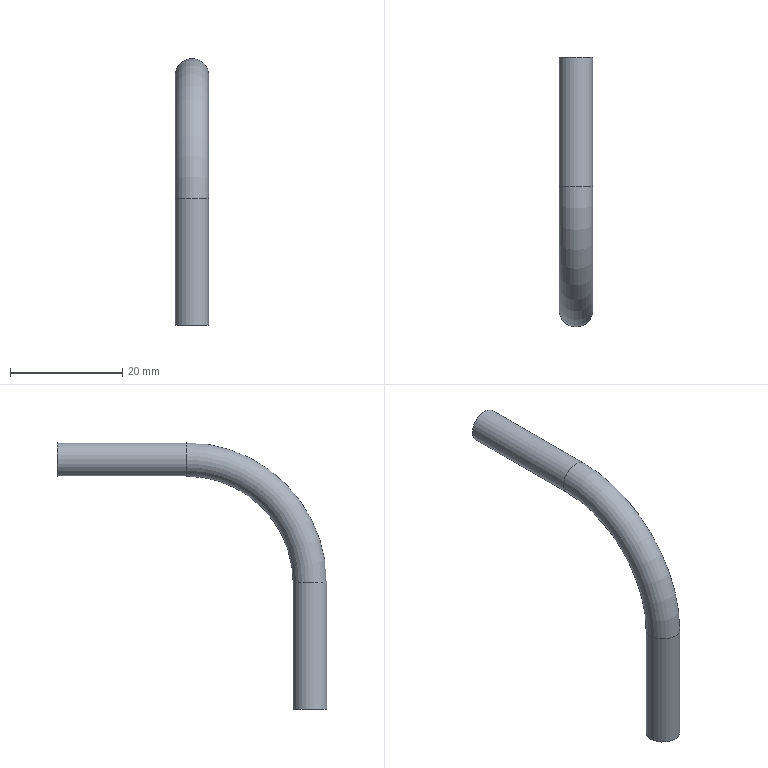Part | STEP file | 1-51.3 | 1 solid | 8 faces | box 6 x 48 x 47.5 mm | volume 691.647 mm3 | cylinder 4 | torus 2 | plane 2 | commonest cylinder face diameters 5 x2 6 x2
STEP:
#1=CARTESIAN_POINT('',(0.,0.,0.));
#2=DIRECTION('',(0.,0.,1.));
#3=DIRECTION('',(1.,0.,0.));
#4=AXIS2_PLACEMENT_3D('',#1,#2,#3);
#5=CARTESIAN_POINT('',(3.,0.,0.));
#6=VERTEX_POINT('',#5);
#7=CARTESIAN_POINT('',(0.,0.,0.));
#8=DIRECTION('',(0.,0.,-1.));
#9=DIRECTION('',(1.,0.,0.));
#10=AXIS2_PLACEMENT_3D('',#7,#8,#9);
#11=CIRCLE('',#10,3.);
#12=CARTESIAN_POINT('',(0.,0.,0.));
#13=DIRECTION('',(0.,0.,1.));
#14=DIRECTION('',(1.,0.,0.));
#15=AXIS2_PLACEMENT_3D('',#12,#13,#14);
#16=CYLINDRICAL_SURFACE('',#15,3.);
#17=CARTESIAN_POINT('',(6.283,0.));
#18=DIRECTION('',(-1.,0.));
#19=VECTOR('',#18,1.);
#20=LINE('',#17,#19);
#21=(GEOMETRIC_REPRESENTATION_CONTEXT(2)PARAMETRIC_REPRESENTATION_CONTEXT()REPRESENTATION_CONTEXT('',''));
#22=DEFINITIONAL_REPRESENTATION('',(#20),#21);
#23=PCURVE('',#16,#22);
#24=CARTESIAN_POINT('',(0.,0.,0.));
#25=DIRECTION('',(0.,0.,-1.));
#26=DIRECTION('',(1.,0.,0.));
#27=AXIS2_PLACEMENT_3D('',#24,#25,#26);
#28=PLANE('',#27);
#29=CARTESIAN_POINT('',(0.,0.));
#30=DIRECTION('',(1.,0.));
#31=AXIS2_PLACEMENT_2D('',#29,#30);
#32=CIRCLE('',#31,3.);
#33=(GEOMETRIC_REPRESENTATION_CONTEXT(2)PARAMETRIC_REPRESENTATION_CONTEXT()REPRESENTATION_CONTEXT('',''));
#34=DEFINITIONAL_REPRESENTATION('',(#32),#33);
#35=PCURVE('',#28,#34);
#36=SURFACE_CURVE('',#11,(#23,#35),.PCURVE_S1.);
#37=EDGE_CURVE('',#6,#6,#36,.T.);
#38=ORIENTED_EDGE('',*,*,#37,.F.);
#39=CARTESIAN_POINT('',(3.,0.,22.5));
#40=VERTEX_POINT('',#39);
#41=CARTESIAN_POINT('',(3.,0.,0.));
#42=DIRECTION('',(0.,0.,1.));
#43=VECTOR('',#42,1.);
#44=LINE('',#41,#43);
#45=CARTESIAN_POINT('',(6.283,0.));
#46=DIRECTION('',(0.,1.));
#47=VECTOR('',#46,1.);
#48=LINE('',#45,#47);
#49=(GEOMETRIC_REPRESENTATION_CONTEXT(2)PARAMETRIC_REPRESENTATION_CONTEXT()REPRESENTATION_CONTEXT('',''));
#50=DEFINITIONAL_REPRESENTATION('',(#48),#49);
#51=PCURVE('',#16,#50);
#52=CARTESIAN_POINT('',(0.,0.));
#53=DIRECTION('',(0.,1.));
#54=VECTOR('',#53,1.);
#55=LINE('',#52,#54);
#56=(GEOMETRIC_REPRESENTATION_CONTEXT(2)PARAMETRIC_REPRESENTATION_CONTEXT()REPRESENTATION_CONTEXT('',''));
#57=DEFINITIONAL_REPRESENTATION('',(#55),#56);
#58=PCURVE('',#16,#57);
#59=SEAM_CURVE('',#44,(#51,#58),.PCURVE_S1.);
#60=EDGE_CURVE('',#6,#40,#59,.T.);
#61=ORIENTED_EDGE('',*,*,#60,.T.);
#62=CARTESIAN_POINT('',(-3.,0.,22.5));
#63=VERTEX_POINT('',#62);
#64=CARTESIAN_POINT('',(0.,0.,22.5));
#65=DIRECTION('',(0.,0.,1.));
#66=DIRECTION('',(-1.,0.,0.));
#67=AXIS2_PLACEMENT_3D('',#64,#65,#66);
#68=CIRCLE('',#67,3.);
#69=CARTESIAN_POINT('',(3.142,22.5));
#70=DIRECTION('',(1.,0.));
#71=VECTOR('',#70,1.);
#72=LINE('',#69,#71);
#73=(GEOMETRIC_REPRESENTATION_CONTEXT(2)PARAMETRIC_REPRESENTATION_CONTEXT()REPRESENTATION_CONTEXT('',''));
#74=DEFINITIONAL_REPRESENTATION('',(#72),#73);
#75=PCURVE('',#16,#74);
#76=CARTESIAN_POINT('',(0.,22.,22.5));
#77=DIRECTION('',(1.,0.,0.));
#78=DIRECTION('',(0.,-1.,0.));
#79=AXIS2_PLACEMENT_3D('',#76,#77,#78);
#80=TOROIDAL_SURFACE('',#79,22.,3.);
#81=CARTESIAN_POINT('',(6.283,-1.571));
#82=DIRECTION('',(0.,1.));
#83=VECTOR('',#82,1.);
#84=LINE('',#81,#83);
#85=(GEOMETRIC_REPRESENTATION_CONTEXT(2)PARAMETRIC_REPRESENTATION_CONTEXT()REPRESENTATION_CONTEXT('',''));
#86=DEFINITIONAL_REPRESENTATION('',(#84),#85);
#87=PCURVE('',#80,#86);
#88=SURFACE_CURVE('',#68,(#75,#87),.PCURVE_S1.);
#89=EDGE_CURVE('',#63,#40,#88,.T.);
#90=ORIENTED_EDGE('',*,*,#89,.F.);
#91=CARTESIAN_POINT('',(0.,0.,22.5));
#92=DIRECTION('',(0.,0.,1.));
#93=DIRECTION('',(1.,0.,0.));
#94=AXIS2_PLACEMENT_3D('',#91,#92,#93);
#95=CIRCLE('',#94,3.);
#96=CARTESIAN_POINT('',(0.,22.5));
#97=DIRECTION('',(1.,0.));
#98=VECTOR('',#97,1.);
#99=LINE('',#96,#98);
#100=(GEOMETRIC_REPRESENTATION_CONTEXT(2)PARAMETRIC_REPRESENTATION_CONTEXT()REPRESENTATION_CONTEXT('',''));
#101=DEFINITIONAL_REPRESENTATION('',(#99),#100);
#102=PCURVE('',#16,#101);
#103=CARTESIAN_POINT('',(6.283,1.571));
#104=DIRECTION('',(0.,1.));
#105=VECTOR('',#104,1.);
#106=LINE('',#103,#105);
#107=(GEOMETRIC_REPRESENTATION_CONTEXT(2)PARAMETRIC_REPRESENTATION_CONTEXT()REPRESENTATION_CONTEXT('',''));
#108=DEFINITIONAL_REPRESENTATION('',(#106),#107);
#109=PCURVE('',#80,#108);
#110=SURFACE_CURVE('',#95,(#102,#109),.PCURVE_S1.);
#111=EDGE_CURVE('',#40,#63,#110,.T.);
#112=ORIENTED_EDGE('',*,*,#111,.F.);
#113=ORIENTED_EDGE('',*,*,#60,.F.);
#114=EDGE_LOOP('',(#38,#61,#90,#112,#113));
#115=FACE_BOUND('',#114,.T.);
#116=ADVANCED_FACE('',(#115),#16,.T.);
#117=ORIENTED_EDGE('',*,*,#89,.T.);
#118=ORIENTED_EDGE('',*,*,#111,.T.);
#119=CARTESIAN_POINT('',(-3.,22.,44.5));
#120=VERTEX_POINT('',#119);
#121=CARTESIAN_POINT('',(-3.,22.,22.5));
#122=DIRECTION('',(-1.,0.,0.));
#123=DIRECTION('',(0.,-1.,0.));
#124=AXIS2_PLACEMENT_3D('',#121,#122,#123);
#125=CIRCLE('',#124,22.);
#126=CARTESIAN_POINT('',(6.283,4.712));
#127=DIRECTION('',(-1.,0.));
#128=VECTOR('',#127,1.);
#129=LINE('',#126,#128);
#130=(GEOMETRIC_REPRESENTATION_CONTEXT(2)PARAMETRIC_REPRESENTATION_CONTEXT()REPRESENTATION_CONTEXT('',''));
#131=DEFINITIONAL_REPRESENTATION('',(#129),#130);
#132=PCURVE('',#80,#131);
#133=CARTESIAN_POINT('',(6.283,-1.571));
#134=DIRECTION('',(-1.,0.));
#135=VECTOR('',#134,1.);
#136=LINE('',#133,#135);
#137=(GEOMETRIC_REPRESENTATION_CONTEXT(2)PARAMETRIC_REPRESENTATION_CONTEXT()REPRESENTATION_CONTEXT('',''));
#138=DEFINITIONAL_REPRESENTATION('',(#136),#137);
#139=PCURVE('',#80,#138);
#140=SEAM_CURVE('',#125,(#132,#139),.PCURVE_S1.);
#141=EDGE_CURVE('',#63,#120,#140,.T.);
#142=ORIENTED_EDGE('',*,*,#141,.T.);
#143=CARTESIAN_POINT('',(3.,22.,44.5));
#144=VERTEX_POINT('',#143);
#145=CARTESIAN_POINT('',(0.,22.,44.5));
#146=DIRECTION('',(0.,-1.,0.));
#147=DIRECTION('',(-1.,0.,0.));
#148=AXIS2_PLACEMENT_3D('',#145,#146,#147);
#149=CIRCLE('',#148,3.);
#150=CARTESIAN_POINT('',(4.712,4.712));
#151=DIRECTION('',(0.,-1.));
#152=VECTOR('',#151,1.);
#153=LINE('',#150,#152);
#154=(GEOMETRIC_REPRESENTATION_CONTEXT(2)PARAMETRIC_REPRESENTATION_CONTEXT()REPRESENTATION_CONTEXT('',''));
#155=DEFINITIONAL_REPRESENTATION('',(#153),#154);
#156=PCURVE('',#80,#155);
#157=CARTESIAN_POINT('',(0.,22.,44.5));
#158=DIRECTION('',(0.,1.,0.));
#159=DIRECTION('',(1.,0.,0.));
#160=AXIS2_PLACEMENT_3D('',#157,#158,#159);
#161=CYLINDRICAL_SURFACE('',#160,3.);
#162=CARTESIAN_POINT('',(3.142,0.));
#163=DIRECTION('',(-1.,0.));
#164=VECTOR('',#163,1.);
#165=LINE('',#162,#164);
#166=(GEOMETRIC_REPRESENTATION_CONTEXT(2)PARAMETRIC_REPRESENTATION_CONTEXT()REPRESENTATION_CONTEXT('',''));
#167=DEFINITIONAL_REPRESENTATION('',(#165),#166);
#168=PCURVE('',#161,#167);
#169=SURFACE_CURVE('',#149,(#156,#168),.PCURVE_S1.);
#170=EDGE_CURVE('',#120,#144,#169,.T.);
#171=ORIENTED_EDGE('',*,*,#170,.T.);
#172=CARTESIAN_POINT('',(0.,22.,44.5));
#173=DIRECTION('',(0.,-1.,0.));
#174=DIRECTION('',(1.,0.,0.));
#175=AXIS2_PLACEMENT_3D('',#172,#173,#174);
#176=CIRCLE('',#175,3.);
#177=CARTESIAN_POINT('',(4.712,1.571));
#178=DIRECTION('',(0.,-1.));
#179=VECTOR('',#178,1.);
#180=LINE('',#177,#179);
#181=(GEOMETRIC_REPRESENTATION_CONTEXT(2)PARAMETRIC_REPRESENTATION_CONTEXT()REPRESENTATION_CONTEXT('',''));
#182=DEFINITIONAL_REPRESENTATION('',(#180),#181);
#183=PCURVE('',#80,#182);
#184=CARTESIAN_POINT('',(6.283,0.));
#185=DIRECTION('',(-1.,0.));
#186=VECTOR('',#185,1.);
#187=LINE('',#184,#186);
#188=(GEOMETRIC_REPRESENTATION_CONTEXT(2)PARAMETRIC_REPRESENTATION_CONTEXT()REPRESENTATION_CONTEXT('',''));
#189=DEFINITIONAL_REPRESENTATION('',(#187),#188);
#190=PCURVE('',#161,#189);
#191=SURFACE_CURVE('',#176,(#183,#190),.PCURVE_S1.);
#192=EDGE_CURVE('',#144,#120,#191,.T.);
#193=ORIENTED_EDGE('',*,*,#192,.T.);
#194=ORIENTED_EDGE('',*,*,#141,.F.);
#195=EDGE_LOOP('',(#117,#118,#142,#171,#193,#194));
#196=FACE_BOUND('',#195,.T.);
#197=ADVANCED_FACE('',(#196),#80,.T.);
#198=ORIENTED_EDGE('',*,*,#170,.F.);
#199=ORIENTED_EDGE('',*,*,#192,.F.);
#200=CARTESIAN_POINT('',(3.,45.,44.5));
#201=VERTEX_POINT('',#200);
#202=CARTESIAN_POINT('',(3.,22.,44.5));
#203=DIRECTION('',(0.,1.,0.));
#204=VECTOR('',#203,1.);
#205=LINE('',#202,#204);
#206=CARTESIAN_POINT('',(6.283,0.));
#207=DIRECTION('',(0.,1.));
#208=VECTOR('',#207,1.);
#209=LINE('',#206,#208);
#210=(GEOMETRIC_REPRESENTATION_CONTEXT(2)PARAMETRIC_REPRESENTATION_CONTEXT()REPRESENTATION_CONTEXT('',''));
#211=DEFINITIONAL_REPRESENTATION('',(#209),#210);
#212=PCURVE('',#161,#211);
#213=CARTESIAN_POINT('',(0.,0.));
#214=DIRECTION('',(0.,1.));
#215=VECTOR('',#214,1.);
#216=LINE('',#213,#215);
#217=(GEOMETRIC_REPRESENTATION_CONTEXT(2)PARAMETRIC_REPRESENTATION_CONTEXT()REPRESENTATION_CONTEXT('',''));
#218=DEFINITIONAL_REPRESENTATION('',(#216),#217);
#219=PCURVE('',#161,#218);
#220=SEAM_CURVE('',#205,(#212,#219),.PCURVE_S1.);
#221=EDGE_CURVE('',#144,#201,#220,.T.);
#222=ORIENTED_EDGE('',*,*,#221,.T.);
#223=CARTESIAN_POINT('',(0.,45.,44.5));
#224=DIRECTION('',(0.,1.,0.));
#225=DIRECTION('',(1.,0.,0.));
#226=AXIS2_PLACEMENT_3D('',#223,#224,#225);
#227=CIRCLE('',#226,3.);
#228=CARTESIAN_POINT('',(0.,23.));
#229=DIRECTION('',(1.,0.));
#230=VECTOR('',#229,1.);
#231=LINE('',#228,#230);
#232=(GEOMETRIC_REPRESENTATION_CONTEXT(2)PARAMETRIC_REPRESENTATION_CONTEXT()REPRESENTATION_CONTEXT('',''));
#233=DEFINITIONAL_REPRESENTATION('',(#231),#232);
#234=PCURVE('',#161,#233);
#235=CARTESIAN_POINT('',(0.,45.,44.5));
#236=DIRECTION('',(0.,1.,0.));
#237=DIRECTION('',(0.,0.,1.));
#238=AXIS2_PLACEMENT_3D('',#235,#236,#237);
#239=PLANE('',#238);
#240=CARTESIAN_POINT('',(0.,0.));
#241=DIRECTION('',(0.,1.));
#242=AXIS2_PLACEMENT_2D('',#240,#241);
#243=CIRCLE('',#242,3.);
#244=(GEOMETRIC_REPRESENTATION_CONTEXT(2)PARAMETRIC_REPRESENTATION_CONTEXT()REPRESENTATION_CONTEXT('',''));
#245=DEFINITIONAL_REPRESENTATION('',(#243),#244);
#246=PCURVE('',#239,#245);
#247=SURFACE_CURVE('',#227,(#234,#246),.PCURVE_S1.);
#248=EDGE_CURVE('',#201,#201,#247,.T.);
#249=ORIENTED_EDGE('',*,*,#248,.F.);
#250=ORIENTED_EDGE('',*,*,#221,.F.);
#251=EDGE_LOOP('',(#198,#199,#222,#249,#250));
#252=FACE_BOUND('',#251,.T.);
#253=ADVANCED_FACE('',(#252),#161,.T.);
#254=ORIENTED_EDGE('',*,*,#37,.T.);
#255=EDGE_LOOP('',(#254));
#256=FACE_BOUND('',#255,.T.);
#257=CARTESIAN_POINT('',(2.5,0.,0.));
#258=VERTEX_POINT('',#257);
#259=CARTESIAN_POINT('',(0.,0.,0.));
#260=DIRECTION('',(0.,0.,-1.));
#261=DIRECTION('',(1.,0.,0.));
#262=AXIS2_PLACEMENT_3D('',#259,#260,#261);
#263=CIRCLE('',#262,2.5);
#264=CARTESIAN_POINT('',(0.,0.));
#265=DIRECTION('',(1.,0.));
#266=AXIS2_PLACEMENT_2D('',#264,#265);
#267=CIRCLE('',#266,2.5);
#268=(GEOMETRIC_REPRESENTATION_CONTEXT(2)PARAMETRIC_REPRESENTATION_CONTEXT()REPRESENTATION_CONTEXT('',''));
#269=DEFINITIONAL_REPRESENTATION('',(#267),#268);
#270=PCURVE('',#28,#269);
#271=CARTESIAN_POINT('',(0.,0.,0.));
#272=DIRECTION('',(0.,0.,1.));
#273=DIRECTION('',(1.,0.,0.));
#274=AXIS2_PLACEMENT_3D('',#271,#272,#273);
#275=CYLINDRICAL_SURFACE('',#274,2.5);
#276=CARTESIAN_POINT('',(6.283,0.));
#277=DIRECTION('',(-1.,0.));
#278=VECTOR('',#277,1.);
#279=LINE('',#276,#278);
#280=(GEOMETRIC_REPRESENTATION_CONTEXT(2)PARAMETRIC_REPRESENTATION_CONTEXT()REPRESENTATION_CONTEXT('',''));
#281=DEFINITIONAL_REPRESENTATION('',(#279),#280);
#282=PCURVE('',#275,#281);
#283=SURFACE_CURVE('',#263,(#270,#282),.PCURVE_S1.);
#284=EDGE_CURVE('',#258,#258,#283,.T.);
#285=ORIENTED_EDGE('',*,*,#284,.F.);
#286=EDGE_LOOP('',(#285));
#287=FACE_BOUND('',#286,.T.);
#288=ADVANCED_FACE('',(#256,#287),#28,.T.);
#289=ORIENTED_EDGE('',*,*,#248,.T.);
#290=EDGE_LOOP('',(#289));
#291=FACE_BOUND('',#290,.T.);
#292=CARTESIAN_POINT('',(2.5,45.,44.5));
#293=VERTEX_POINT('',#292);
#294=CARTESIAN_POINT('',(0.,45.,44.5));
#295=DIRECTION('',(0.,1.,0.));
#296=DIRECTION('',(1.,0.,0.));
#297=AXIS2_PLACEMENT_3D('',#294,#295,#296);
#298=CIRCLE('',#297,2.5);
#299=CARTESIAN_POINT('',(0.,0.));
#300=DIRECTION('',(0.,1.));
#301=AXIS2_PLACEMENT_2D('',#299,#300);
#302=CIRCLE('',#301,2.5);
#303=(GEOMETRIC_REPRESENTATION_CONTEXT(2)PARAMETRIC_REPRESENTATION_CONTEXT()REPRESENTATION_CONTEXT('',''));
#304=DEFINITIONAL_REPRESENTATION('',(#302),#303);
#305=PCURVE('',#239,#304);
#306=CARTESIAN_POINT('',(0.,22.,44.5));
#307=DIRECTION('',(0.,1.,0.));
#308=DIRECTION('',(1.,0.,0.));
#309=AXIS2_PLACEMENT_3D('',#306,#307,#308);
#310=CYLINDRICAL_SURFACE('',#309,2.5);
#311=CARTESIAN_POINT('',(0.,23.));
#312=DIRECTION('',(1.,0.));
#313=VECTOR('',#312,1.);
#314=LINE('',#311,#313);
#315=(GEOMETRIC_REPRESENTATION_CONTEXT(2)PARAMETRIC_REPRESENTATION_CONTEXT()REPRESENTATION_CONTEXT('',''));
#316=DEFINITIONAL_REPRESENTATION('',(#314),#315);
#317=PCURVE('',#310,#316);
#318=SURFACE_CURVE('',#298,(#305,#317),.PCURVE_S1.);
#319=EDGE_CURVE('',#293,#293,#318,.T.);
#320=ORIENTED_EDGE('',*,*,#319,.F.);
#321=EDGE_LOOP('',(#320));
#322=FACE_BOUND('',#321,.T.);
#323=ADVANCED_FACE('',(#291,#322),#239,.T.);
#324=ORIENTED_EDGE('',*,*,#284,.F.);
#325=CARTESIAN_POINT('',(2.5,0.,22.5));
#326=VERTEX_POINT('',#325);
#327=CARTESIAN_POINT('',(2.5,0.,0.));
#328=DIRECTION('',(0.,0.,1.));
#329=VECTOR('',#328,1.);
#330=LINE('',#327,#329);
#331=CARTESIAN_POINT('',(6.283,0.));
#332=DIRECTION('',(0.,1.));
#333=VECTOR('',#332,1.);
#334=LINE('',#331,#333);
#335=(GEOMETRIC_REPRESENTATION_CONTEXT(2)PARAMETRIC_REPRESENTATION_CONTEXT()REPRESENTATION_CONTEXT('',''));
#336=DEFINITIONAL_REPRESENTATION('',(#334),#335);
#337=PCURVE('',#275,#336);
#338=CARTESIAN_POINT('',(0.,0.));
#339=DIRECTION('',(0.,1.));
#340=VECTOR('',#339,1.);
#341=LINE('',#338,#340);
#342=(GEOMETRIC_REPRESENTATION_CONTEXT(2)PARAMETRIC_REPRESENTATION_CONTEXT()REPRESENTATION_CONTEXT('',''));
#343=DEFINITIONAL_REPRESENTATION('',(#341),#342);
#344=PCURVE('',#275,#343);
#345=SEAM_CURVE('',#330,(#337,#344),.PCURVE_S1.);
#346=EDGE_CURVE('',#258,#326,#345,.T.);
#347=ORIENTED_EDGE('',*,*,#346,.T.);
#348=CARTESIAN_POINT('',(-2.5,0.,22.5));
#349=VERTEX_POINT('',#348);
#350=CARTESIAN_POINT('',(0.,0.,22.5));
#351=DIRECTION('',(0.,0.,1.));
#352=DIRECTION('',(-1.,0.,0.));
#353=AXIS2_PLACEMENT_3D('',#350,#351,#352);
#354=CIRCLE('',#353,2.5);
#355=CARTESIAN_POINT('',(3.142,22.5));
#356=DIRECTION('',(1.,0.));
#357=VECTOR('',#356,1.);
#358=LINE('',#355,#357);
#359=(GEOMETRIC_REPRESENTATION_CONTEXT(2)PARAMETRIC_REPRESENTATION_CONTEXT()REPRESENTATION_CONTEXT('',''));
#360=DEFINITIONAL_REPRESENTATION('',(#358),#359);
#361=PCURVE('',#275,#360);
#362=CARTESIAN_POINT('',(0.,22.,22.5));
#363=DIRECTION('',(1.,0.,0.));
#364=DIRECTION('',(0.,-1.,0.));
#365=AXIS2_PLACEMENT_3D('',#362,#363,#364);
#366=TOROIDAL_SURFACE('',#365,22.,2.5);
#367=CARTESIAN_POINT('',(6.283,-1.571));
#368=DIRECTION('',(0.,1.));
#369=VECTOR('',#368,1.);
#370=LINE('',#367,#369);
#371=(GEOMETRIC_REPRESENTATION_CONTEXT(2)PARAMETRIC_REPRESENTATION_CONTEXT()REPRESENTATION_CONTEXT('',''));
#372=DEFINITIONAL_REPRESENTATION('',(#370),#371);
#373=PCURVE('',#366,#372);
#374=SURFACE_CURVE('',#354,(#361,#373),.PCURVE_S1.);
#375=EDGE_CURVE('',#349,#326,#374,.T.);
#376=ORIENTED_EDGE('',*,*,#375,.F.);
#377=CARTESIAN_POINT('',(0.,0.,22.5));
#378=DIRECTION('',(0.,0.,1.));
#379=DIRECTION('',(1.,0.,0.));
#380=AXIS2_PLACEMENT_3D('',#377,#378,#379);
#381=CIRCLE('',#380,2.5);
#382=CARTESIAN_POINT('',(0.,22.5));
#383=DIRECTION('',(1.,0.));
#384=VECTOR('',#383,1.);
#385=LINE('',#382,#384);
#386=(GEOMETRIC_REPRESENTATION_CONTEXT(2)PARAMETRIC_REPRESENTATION_CONTEXT()REPRESENTATION_CONTEXT('',''));
#387=DEFINITIONAL_REPRESENTATION('',(#385),#386);
#388=PCURVE('',#275,#387);
#389=CARTESIAN_POINT('',(6.283,1.571));
#390=DIRECTION('',(0.,1.));
#391=VECTOR('',#390,1.);
#392=LINE('',#389,#391);
#393=(GEOMETRIC_REPRESENTATION_CONTEXT(2)PARAMETRIC_REPRESENTATION_CONTEXT()REPRESENTATION_CONTEXT('',''));
#394=DEFINITIONAL_REPRESENTATION('',(#392),#393);
#395=PCURVE('',#366,#394);
#396=SURFACE_CURVE('',#381,(#388,#395),.PCURVE_S1.);
#397=EDGE_CURVE('',#326,#349,#396,.T.);
#398=ORIENTED_EDGE('',*,*,#397,.F.);
#399=ORIENTED_EDGE('',*,*,#346,.F.);
#400=EDGE_LOOP('',(#324,#347,#376,#398,#399));
#401=FACE_BOUND('',#400,.F.);
#402=ADVANCED_FACE('',(#401),#275,.F.);
#403=ORIENTED_EDGE('',*,*,#375,.T.);
#404=ORIENTED_EDGE('',*,*,#397,.T.);
#405=CARTESIAN_POINT('',(-2.5,22.,44.5));
#406=VERTEX_POINT('',#405);
#407=CARTESIAN_POINT('',(-2.5,22.,22.5));
#408=DIRECTION('',(-1.,0.,0.));
#409=DIRECTION('',(0.,-1.,0.));
#410=AXIS2_PLACEMENT_3D('',#407,#408,#409);
#411=CIRCLE('',#410,22.);
#412=CARTESIAN_POINT('',(6.283,4.712));
#413=DIRECTION('',(-1.,0.));
#414=VECTOR('',#413,1.);
#415=LINE('',#412,#414);
#416=(GEOMETRIC_REPRESENTATION_CONTEXT(2)PARAMETRIC_REPRESENTATION_CONTEXT()REPRESENTATION_CONTEXT('',''));
#417=DEFINITIONAL_REPRESENTATION('',(#415),#416);
#418=PCURVE('',#366,#417);
#419=CARTESIAN_POINT('',(6.283,-1.571));
#420=DIRECTION('',(-1.,0.));
#421=VECTOR('',#420,1.);
#422=LINE('',#419,#421);
#423=(GEOMETRIC_REPRESENTATION_CONTEXT(2)PARAMETRIC_REPRESENTATION_CONTEXT()REPRESENTATION_CONTEXT('',''));
#424=DEFINITIONAL_REPRESENTATION('',(#422),#423);
#425=PCURVE('',#366,#424);
#426=SEAM_CURVE('',#411,(#418,#425),.PCURVE_S1.);
#427=EDGE_CURVE('',#349,#406,#426,.T.);
#428=ORIENTED_EDGE('',*,*,#427,.T.);
#429=CARTESIAN_POINT('',(2.5,22.,44.5));
#430=VERTEX_POINT('',#429);
#431=CARTESIAN_POINT('',(0.,22.,44.5));
#432=DIRECTION('',(0.,-1.,0.));
#433=DIRECTION('',(-1.,0.,0.));
#434=AXIS2_PLACEMENT_3D('',#431,#432,#433);
#435=CIRCLE('',#434,2.5);
#436=CARTESIAN_POINT('',(4.712,4.712));
#437=DIRECTION('',(0.,-1.));
#438=VECTOR('',#437,1.);
#439=LINE('',#436,#438);
#440=(GEOMETRIC_REPRESENTATION_CONTEXT(2)PARAMETRIC_REPRESENTATION_CONTEXT()REPRESENTATION_CONTEXT('',''));
#441=DEFINITIONAL_REPRESENTATION('',(#439),#440);
#442=PCURVE('',#366,#441);
#443=CARTESIAN_POINT('',(3.142,0.));
#444=DIRECTION('',(-1.,0.));
#445=VECTOR('',#444,1.);
#446=LINE('',#443,#445);
#447=(GEOMETRIC_REPRESENTATION_CONTEXT(2)PARAMETRIC_REPRESENTATION_CONTEXT()REPRESENTATION_CONTEXT('',''));
#448=DEFINITIONAL_REPRESENTATION('',(#446),#447);
#449=PCURVE('',#310,#448);
#450=SURFACE_CURVE('',#435,(#442,#449),.PCURVE_S1.);
#451=EDGE_CURVE('',#406,#430,#450,.T.);
#452=ORIENTED_EDGE('',*,*,#451,.T.);
#453=CARTESIAN_POINT('',(0.,22.,44.5));
#454=DIRECTION('',(0.,-1.,0.));
#455=DIRECTION('',(1.,0.,0.));
#456=AXIS2_PLACEMENT_3D('',#453,#454,#455);
#457=CIRCLE('',#456,2.5);
#458=CARTESIAN_POINT('',(4.712,1.571));
#459=DIRECTION('',(0.,-1.));
#460=VECTOR('',#459,1.);
#461=LINE('',#458,#460);
#462=(GEOMETRIC_REPRESENTATION_CONTEXT(2)PARAMETRIC_REPRESENTATION_CONTEXT()REPRESENTATION_CONTEXT('',''));
#463=DEFINITIONAL_REPRESENTATION('',(#461),#462);
#464=PCURVE('',#366,#463);
#465=CARTESIAN_POINT('',(6.283,0.));
#466=DIRECTION('',(-1.,0.));
#467=VECTOR('',#466,1.);
#468=LINE('',#465,#467);
#469=(GEOMETRIC_REPRESENTATION_CONTEXT(2)PARAMETRIC_REPRESENTATION_CONTEXT()REPRESENTATION_CONTEXT('',''));
#470=DEFINITIONAL_REPRESENTATION('',(#468),#469);
#471=PCURVE('',#310,#470);
#472=SURFACE_CURVE('',#457,(#464,#471),.PCURVE_S1.);
#473=EDGE_CURVE('',#430,#406,#472,.T.);
#474=ORIENTED_EDGE('',*,*,#473,.T.);
#475=ORIENTED_EDGE('',*,*,#427,.F.);
#476=EDGE_LOOP('',(#403,#404,#428,#452,#474,#475));
#477=FACE_BOUND('',#476,.F.);
#478=ADVANCED_FACE('',(#477),#366,.F.);
#479=ORIENTED_EDGE('',*,*,#451,.F.);
#480=ORIENTED_EDGE('',*,*,#473,.F.);
#481=CARTESIAN_POINT('',(2.5,22.,44.5));
#482=DIRECTION('',(0.,1.,0.));
#483=VECTOR('',#482,1.);
#484=LINE('',#481,#483);
#485=CARTESIAN_POINT('',(6.283,0.));
#486=DIRECTION('',(0.,1.));
#487=VECTOR('',#486,1.);
#488=LINE('',#485,#487);
#489=(GEOMETRIC_REPRESENTATION_CONTEXT(2)PARAMETRIC_REPRESENTATION_CONTEXT()REPRESENTATION_CONTEXT('',''));
#490=DEFINITIONAL_REPRESENTATION('',(#488),#489);
#491=PCURVE('',#310,#490);
#492=CARTESIAN_POINT('',(0.,0.));
#493=DIRECTION('',(0.,1.));
#494=VECTOR('',#493,1.);
#495=LINE('',#492,#494);
#496=(GEOMETRIC_REPRESENTATION_CONTEXT(2)PARAMETRIC_REPRESENTATION_CONTEXT()REPRESENTATION_CONTEXT('',''));
#497=DEFINITIONAL_REPRESENTATION('',(#495),#496);
#498=PCURVE('',#310,#497);
#499=SEAM_CURVE('',#484,(#491,#498),.PCURVE_S1.);
#500=EDGE_CURVE('',#430,#293,#499,.T.);
#501=ORIENTED_EDGE('',*,*,#500,.T.);
#502=ORIENTED_EDGE('',*,*,#319,.F.);
#503=ORIENTED_EDGE('',*,*,#500,.F.);
#504=EDGE_LOOP('',(#479,#480,#501,#502,#503));
#505=FACE_BOUND('',#504,.F.);
#506=ADVANCED_FACE('',(#505),#310,.F.);
#507=CLOSED_SHELL('',(#116,#197,#253,#288,#323,#402,#478,#506));
#508=MANIFOLD_SOLID_BREP('',#507);
#509=(LENGTH_UNIT()NAMED_UNIT(*)SI_UNIT(.MILLI.,.METRE.));
#510=UNCERTAINTY_MEASURE_WITH_UNIT(LENGTH_MEASURE(0.0000001),#509,'','');
#511=(NAMED_UNIT(*)PLANE_ANGLE_UNIT()SI_UNIT($,.RADIAN.));
#512=(NAMED_UNIT(*)SI_UNIT($,.STERADIAN.)SOLID_ANGLE_UNIT());
#513=(GEOMETRIC_REPRESENTATION_CONTEXT(3)GLOBAL_UNCERTAINTY_ASSIGNED_CONTEXT((#510))GLOBAL_UNIT_ASSIGNED_CONTEXT((#509,#511,#512))REPRESENTATION_CONTEXT('',''));
#514=ADVANCED_BREP_SHAPE_REPRESENTATION('',(#4,#508),#513);